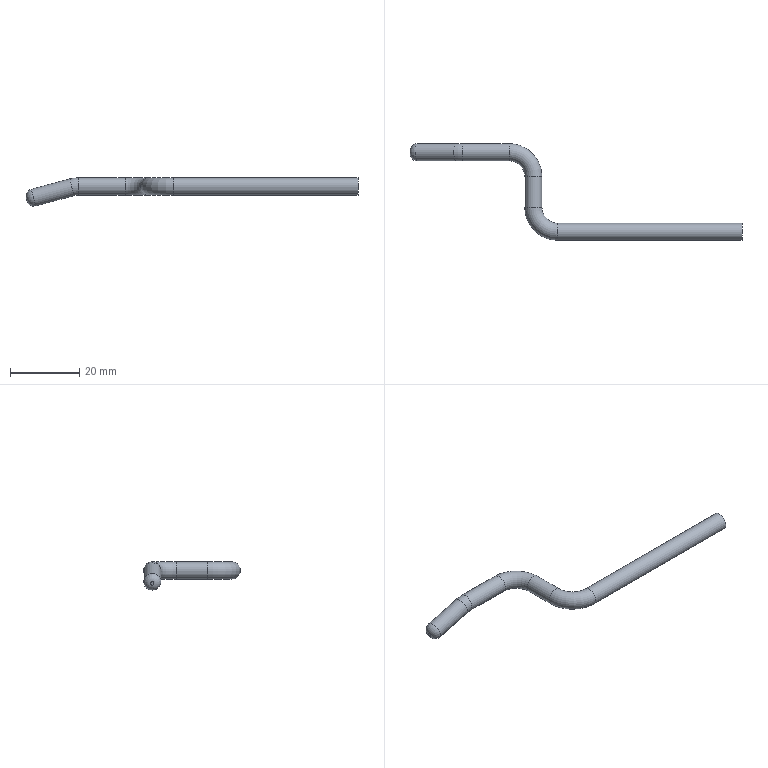Part | NX | features solid 2 | 1 solid | 10 faces | box 96.06 x 28 x 8.217 mm | volume 2214 mm3 | cylinder 4 | torus 4 | plane 2 | commonest cylinder face diameters 5 x4
STEP:
#1=CARTESIAN_POINT('',(386.422,36.,-5.819));
#2=VERTEX_POINT('',#1);
#3=CARTESIAN_POINT('',(387.069,36.,-8.234));
#4=DIRECTION('',(-0.9659,0.,-0.2588));
#5=DIRECTION('',(-0.2588,0.,0.9659));
#6=AXIS2_PLACEMENT_3D('',#3,#4,#5);
#7=CIRCLE('',#6,2.5);
#8=EDGE_CURVE('',#2,#2,#7,.F.);
#9=ORIENTED_EDGE('',*,*,#8,.T.);
#10=EDGE_LOOP('',(#9));
#11=FACE_BOUND('',#10,.T.);
#12=CARTESIAN_POINT('',(397.601,36.,-2.824));
#13=VERTEX_POINT('',#12);
#14=CARTESIAN_POINT('',(398.248,36.,-5.239));
#15=DIRECTION('',(-0.9659,0.,-0.2588));
#16=DIRECTION('',(-0.2588,0.,0.9659));
#17=AXIS2_PLACEMENT_3D('',#14,#15,#16);
#18=CIRCLE('',#17,2.5);
#19=EDGE_CURVE('',#13,#13,#18,.T.);
#20=ORIENTED_EDGE('',*,*,#19,.T.);
#21=EDGE_LOOP('',(#20));
#22=FACE_BOUND('',#21,.T.);
#23=CARTESIAN_POINT('',(398.248,36.,-5.239));
#24=DIRECTION('',(-0.9659,0.,-0.2588));
#25=DIRECTION('',(-0.2588,0.,0.9659));
#26=AXIS2_PLACEMENT_3D('',#23,#24,#25);
#27=CYLINDRICAL_SURFACE('',#26,2.5);
#28=ADVANCED_FACE('',(#11,#22),#27,.T.);
#29=CARTESIAN_POINT('',(400.06,36.,-2.5));
#30=VERTEX_POINT('',#29);
#31=CARTESIAN_POINT('',(400.06,36.,-5.));
#32=DIRECTION('',(-1.,0.,0.));
#33=DIRECTION('',(0.,0.,1.));
#34=AXIS2_PLACEMENT_3D('',#31,#32,#33);
#35=CIRCLE('',#34,2.5);
#36=EDGE_CURVE('',#30,#30,#35,.T.);
#37=ORIENTED_EDGE('',*,*,#36,.T.);
#38=EDGE_LOOP('',(#37));
#39=FACE_BOUND('',#38,.T.);
#40=ORIENTED_EDGE('',*,*,#19,.F.);
#41=EDGE_LOOP('',(#40));
#42=FACE_BOUND('',#41,.T.);
#43=CARTESIAN_POINT('',(400.06,36.,-12.));
#44=DIRECTION('',(0.,-1.,0.));
#45=DIRECTION('',(0.,0.,-1.));
#46=AXIS2_PLACEMENT_3D('',#43,#44,#45);
#47=TOROIDAL_SURFACE('',#46,7.,2.5);
#48=ADVANCED_FACE('',(#39,#42),#47,.T.);
#49=CARTESIAN_POINT('',(413.633,36.,-2.5));
#50=VERTEX_POINT('',#49);
#51=CARTESIAN_POINT('',(413.633,36.,-5.));
#52=DIRECTION('',(-1.,0.,0.));
#53=DIRECTION('',(0.,0.,1.));
#54=AXIS2_PLACEMENT_3D('',#51,#52,#53);
#55=CIRCLE('',#54,2.5);
#56=EDGE_CURVE('',#50,#50,#55,.T.);
#57=ORIENTED_EDGE('',*,*,#56,.T.);
#58=EDGE_LOOP('',(#57));
#59=FACE_BOUND('',#58,.T.);
#60=ORIENTED_EDGE('',*,*,#36,.F.);
#61=EDGE_LOOP('',(#60));
#62=FACE_BOUND('',#61,.T.);
#63=CARTESIAN_POINT('',(413.633,36.,-5.));
#64=DIRECTION('',(-1.,0.,0.));
#65=DIRECTION('',(0.,0.,1.));
#66=AXIS2_PLACEMENT_3D('',#63,#64,#65);
#67=CYLINDRICAL_SURFACE('',#66,2.5);
#68=ADVANCED_FACE('',(#59,#62),#67,.T.);
#69=CARTESIAN_POINT('',(420.633,29.,-2.5));
#70=VERTEX_POINT('',#69);
#71=CARTESIAN_POINT('',(420.633,29.,-5.));
#72=DIRECTION('',(0.,1.,0.));
#73=DIRECTION('',(0.,0.,1.));
#74=AXIS2_PLACEMENT_3D('',#71,#72,#73);
#75=CIRCLE('',#74,2.5);
#76=EDGE_CURVE('',#70,#70,#75,.T.);
#77=ORIENTED_EDGE('',*,*,#76,.T.);
#78=EDGE_LOOP('',(#77));
#79=FACE_BOUND('',#78,.T.);
#80=ORIENTED_EDGE('',*,*,#56,.F.);
#81=EDGE_LOOP('',(#80));
#82=FACE_BOUND('',#81,.T.);
#83=CARTESIAN_POINT('',(413.633,29.,-5.));
#84=DIRECTION('',(0.,0.,1.));
#85=DIRECTION('',(1.,0.,0.));
#86=AXIS2_PLACEMENT_3D('',#83,#84,#85);
#87=TOROIDAL_SURFACE('',#86,7.,2.5);
#88=ADVANCED_FACE('',(#79,#82),#87,.T.);
#89=CARTESIAN_POINT('',(420.633,20.,-2.5));
#90=VERTEX_POINT('',#89);
#91=CARTESIAN_POINT('',(420.633,20.,-5.));
#92=DIRECTION('',(0.,1.,0.));
#93=DIRECTION('',(0.,0.,1.));
#94=AXIS2_PLACEMENT_3D('',#91,#92,#93);
#95=CIRCLE('',#94,2.5);
#96=EDGE_CURVE('',#90,#90,#95,.T.);
#97=ORIENTED_EDGE('',*,*,#96,.T.);
#98=EDGE_LOOP('',(#97));
#99=FACE_BOUND('',#98,.T.);
#100=ORIENTED_EDGE('',*,*,#76,.F.);
#101=EDGE_LOOP('',(#100));
#102=FACE_BOUND('',#101,.T.);
#103=CARTESIAN_POINT('',(420.633,20.,-5.));
#104=DIRECTION('',(0.,1.,0.));
#105=DIRECTION('',(0.,0.,1.));
#106=AXIS2_PLACEMENT_3D('',#103,#104,#105);
#107=CYLINDRICAL_SURFACE('',#106,2.5);
#108=ADVANCED_FACE('',(#99,#102),#107,.T.);
#109=CARTESIAN_POINT('',(427.633,13.,-2.5));
#110=VERTEX_POINT('',#109);
#111=CARTESIAN_POINT('',(427.633,13.,-5.));
#112=DIRECTION('',(-1.,0.,0.));
#113=DIRECTION('',(0.,0.,1.));
#114=AXIS2_PLACEMENT_3D('',#111,#112,#113);
#115=CIRCLE('',#114,2.5);
#116=EDGE_CURVE('',#110,#110,#115,.T.);
#117=ORIENTED_EDGE('',*,*,#116,.T.);
#118=EDGE_LOOP('',(#117));
#119=FACE_BOUND('',#118,.T.);
#120=ORIENTED_EDGE('',*,*,#96,.F.);
#121=EDGE_LOOP('',(#120));
#122=FACE_BOUND('',#121,.T.);
#123=CARTESIAN_POINT('',(427.633,20.,-5.));
#124=DIRECTION('',(0.,0.,-1.));
#125=DIRECTION('',(-1.,0.,0.));
#126=AXIS2_PLACEMENT_3D('',#123,#124,#125);
#127=TOROIDAL_SURFACE('',#126,7.,2.5);
#128=ADVANCED_FACE('',(#119,#122),#127,.T.);
#129=ORIENTED_EDGE('',*,*,#116,.F.);
#130=EDGE_LOOP('',(#129));
#131=FACE_BOUND('',#130,.T.);
#132=CARTESIAN_POINT('',(481.,13.,-2.5));
#133=VERTEX_POINT('',#132);
#134=CARTESIAN_POINT('',(481.,13.,-5.));
#135=DIRECTION('',(-1.,0.,0.));
#136=DIRECTION('',(0.,0.,1.));
#137=AXIS2_PLACEMENT_3D('',#134,#135,#136);
#138=CIRCLE('',#137,2.5);
#139=EDGE_CURVE('',#133,#133,#138,.T.);
#140=ORIENTED_EDGE('',*,*,#139,.T.);
#141=EDGE_LOOP('',(#140));
#142=FACE_BOUND('',#141,.T.);
#143=CARTESIAN_POINT('',(427.633,13.,-5.));
#144=DIRECTION('',(1.,0.,0.));
#145=DIRECTION('',(0.,0.,-1.));
#146=AXIS2_PLACEMENT_3D('',#143,#144,#145);
#147=CYLINDRICAL_SURFACE('',#146,2.5);
#148=ADVANCED_FACE('',(#131,#142),#147,.T.);
#149=CARTESIAN_POINT('',(385.008,36.,-8.269));
#150=VERTEX_POINT('',#149);
#151=CARTESIAN_POINT('',(385.137,36.,-8.752));
#152=DIRECTION('',(-0.9659,0.,-0.2588));
#153=DIRECTION('',(-0.2588,0.,0.9659));
#154=AXIS2_PLACEMENT_3D('',#151,#152,#153);
#155=CIRCLE('',#154,0.5);
#156=EDGE_CURVE('',#150,#150,#155,.T.);
#157=ORIENTED_EDGE('',*,*,#156,.T.);
#158=EDGE_LOOP('',(#157));
#159=FACE_BOUND('',#158,.T.);
#160=CARTESIAN_POINT('',(385.137,36.,-8.752));
#161=DIRECTION('',(-0.9659,0.,-0.2588));
#162=DIRECTION('',(-0.2588,0.,0.9659));
#163=AXIS2_PLACEMENT_3D('',#160,#161,#162);
#164=PLANE('',#163);
#165=ADVANCED_FACE('',(#159),#164,.T.);
#166=ORIENTED_EDGE('',*,*,#139,.F.);
#167=EDGE_LOOP('',(#166));
#168=FACE_BOUND('',#167,.T.);
#169=CARTESIAN_POINT('',(481.,13.,-5.));
#170=DIRECTION('',(-1.,0.,0.));
#171=DIRECTION('',(0.,0.,1.));
#172=AXIS2_PLACEMENT_3D('',#169,#170,#171);
#173=PLANE('',#172);
#174=ADVANCED_FACE('',(#168),#173,.F.);
#175=ORIENTED_EDGE('',*,*,#8,.F.);
#176=EDGE_LOOP('',(#175));
#177=FACE_BOUND('',#176,.T.);
#178=ORIENTED_EDGE('',*,*,#156,.F.);
#179=EDGE_LOOP('',(#178));
#180=FACE_BOUND('',#179,.T.);
#181=CARTESIAN_POINT('',(387.069,36.,-8.234));
#182=DIRECTION('',(-0.9659,0.,-0.2588));
#183=DIRECTION('',(-0.2588,0.,0.9659));
#184=AXIS2_PLACEMENT_3D('',#181,#182,#183);
#185=DEGENERATE_TOROIDAL_SURFACE('',#184,0.5,2.,.T.);
#186=ADVANCED_FACE('',(#177,#180),#185,.T.);
#187=CLOSED_SHELL('',(#28,#48,#68,#88,#108,#128,#148,#165,#174,#186));
#188=MANIFOLD_SOLID_BREP('',#187);
#189=(LENGTH_UNIT()NAMED_UNIT(*)SI_UNIT(.MILLI.,.METRE.));
#190=UNCERTAINTY_MEASURE_WITH_UNIT(LENGTH_MEASURE(0.00001),#189,'','');
#191=(NAMED_UNIT(*)PLANE_ANGLE_UNIT()SI_UNIT($,.RADIAN.));
#192=(NAMED_UNIT(*)SI_UNIT($,.STERADIAN.)SOLID_ANGLE_UNIT());
#193=(GEOMETRIC_REPRESENTATION_CONTEXT(3)GLOBAL_UNCERTAINTY_ASSIGNED_CONTEXT((#190))GLOBAL_UNIT_ASSIGNED_CONTEXT((#189,#191,#192))REPRESENTATION_CONTEXT('',''));
#194=ADVANCED_BREP_SHAPE_REPRESENTATION('',(#188),#193);